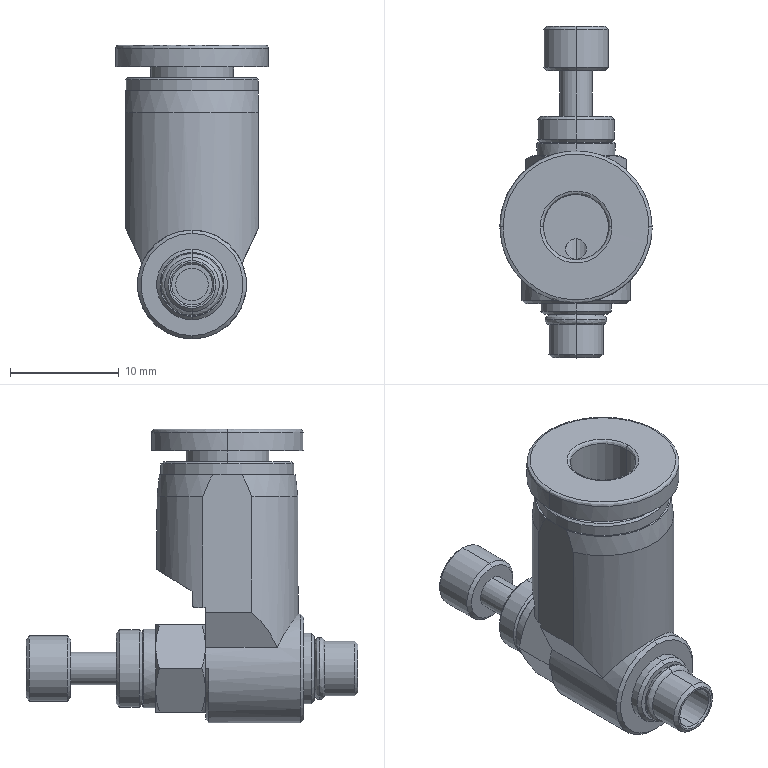Part | STEP file | KZB668-06-M5-668 | 1 solid | 108 faces | box 14 x 30.5 x 27 mm | volume 2988 mm3 | cone 35 | cylinder 33 | plane 32 | spline 8 | commonest cylinder face diameters 3 x4 6 x4 1.9 x2 3.75 x2 4.2 x2 5 x2